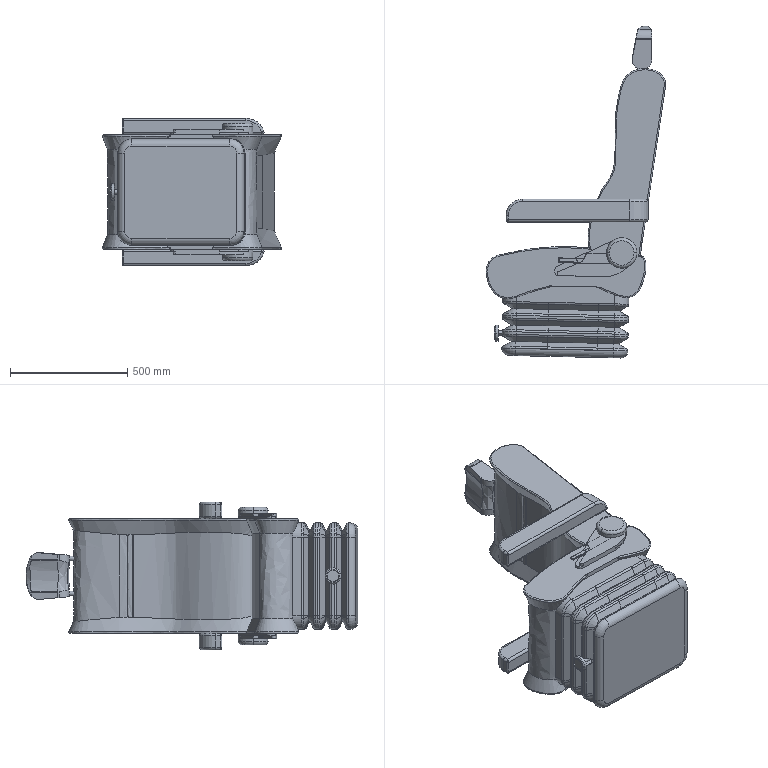Part | SolidWorks | 3 solids | 528 faces | box 766.626 x 1417 x 630 mm | volume 182133754 mm3 | plane 172 | cylinder 169 | torus 64 | spline 53 | cone 50 | sphere 20 | commonest cylinder face diameters 20 x74 4 x24 120 x16 24 x4 60 x4 128.667 x4